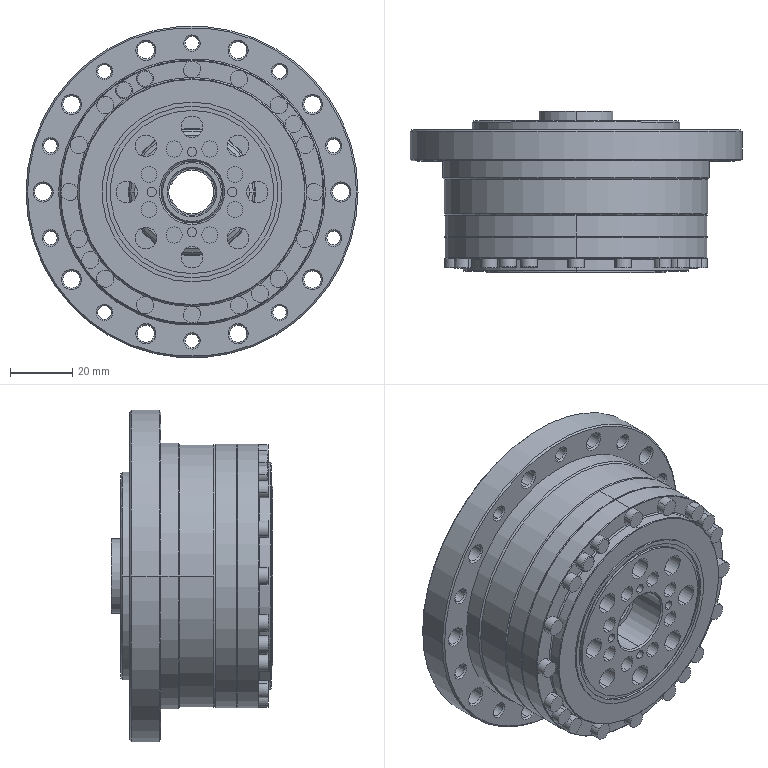Part | SolidWorks | features BaseBody 45 | 45 solids | 853 faces | box 107 x 52 x 107 mm | volume 219965 mm3 | cylinder 393 | cone 210 | plane 136 | sphere 68 | torus 42 | spline 4 | commonest cylinder face diameters 3.5 x72 5.5 x60 6 x52 2.459 x40 3 x16 4.351 x16